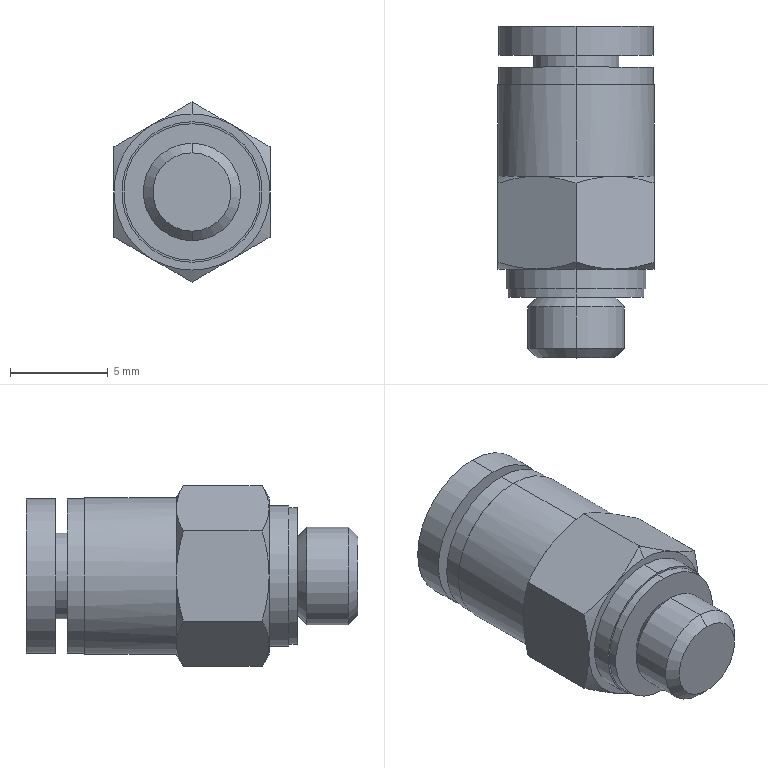Part | SolidWorks | features BaseBody 1 | 1 solid | 49 faces | box 8 x 17 x 9.238 mm | volume 564.577 mm3 | cone 18 | cylinder 16 | plane 15 | commonest cylinder face diameters 7.9 x4 4.2 x2 4.4 x2 5 x2 7 x2 7.2 x2
STEP:
#1=CARTESIAN_POINT('',(0.,1.2,-2.1));
#2=VERTEX_POINT('',#1);
#3=CARTESIAN_POINT('',(0.,1.2,2.1));
#4=VERTEX_POINT('',#3);
#5=CARTESIAN_POINT('',(0.,1.2,0.));
#6=DIRECTION('',(0.,1.,0.));
#7=DIRECTION('',(0.,0.,1.));
#8=AXIS2_PLACEMENT_3D('',#5,#6,#7);
#9=CIRCLE('',#8,2.1);
#10=EDGE_CURVE('',#2,#4,#9,.T.);
#11=ORIENTED_EDGE('',*,*,#10,.F.);
#12=CARTESIAN_POINT('',(0.,13.9,-2.1));
#13=VERTEX_POINT('',#12);
#14=CARTESIAN_POINT('',(0.,7.55,-2.1));
#15=DIRECTION('',(0.,1.,0.));
#16=VECTOR('',#15,1000.);
#17=LINE('',#14,#16);
#18=EDGE_CURVE('',#2,#13,#17,.T.);
#19=ORIENTED_EDGE('',*,*,#18,.T.);
#20=CARTESIAN_POINT('',(0.,13.9,2.1));
#21=VERTEX_POINT('',#20);
#22=CARTESIAN_POINT('',(0.,13.9,0.));
#23=DIRECTION('',(0.,-1.,0.));
#24=DIRECTION('',(0.,0.,1.));
#25=AXIS2_PLACEMENT_3D('',#22,#23,#24);
#26=CIRCLE('',#25,2.1);
#27=EDGE_CURVE('',#21,#13,#26,.T.);
#28=ORIENTED_EDGE('',*,*,#27,.F.);
#29=CARTESIAN_POINT('',(0.,7.55,2.1));
#30=DIRECTION('',(0.,1.,0.));
#31=VECTOR('',#30,1000.);
#32=LINE('',#29,#31);
#33=EDGE_CURVE('',#4,#21,#32,.T.);
#34=ORIENTED_EDGE('',*,*,#33,.F.);
#35=EDGE_LOOP('',(#11,#19,#28,#34));
#36=FACE_OUTER_BOUND('',#35,.T.);
#37=CARTESIAN_POINT('',(0.,7.55,0.));
#38=DIRECTION('',(0.,1.,0.));
#39=DIRECTION('',(0.,0.,1.));
#40=AXIS2_PLACEMENT_3D('',#37,#38,#39);
#41=CYLINDRICAL_SURFACE('',#40,2.1);
#42=ADVANCED_FACE('',(#36),#41,.F.);
#43=CARTESIAN_POINT('',(0.,12.4,3.95));
#44=VERTEX_POINT('',#43);
#45=CARTESIAN_POINT('',(0.,12.4,-3.95));
#46=VERTEX_POINT('',#45);
#47=CARTESIAN_POINT('',(0.,12.4,0.));
#48=DIRECTION('',(0.,1.,0.));
#49=DIRECTION('',(0.,0.,1.));
#50=AXIS2_PLACEMENT_3D('',#47,#48,#49);
#51=CIRCLE('',#50,3.95);
#52=EDGE_CURVE('',#44,#46,#51,.T.);
#53=ORIENTED_EDGE('',*,*,#52,.T.);
#54=CARTESIAN_POINT('',(0.,13.9,-3.95));
#55=VERTEX_POINT('',#54);
#56=CARTESIAN_POINT('',(0.,13.15,-3.95));
#57=DIRECTION('',(0.,1.,0.));
#58=VECTOR('',#57,1000.);
#59=LINE('',#56,#58);
#60=EDGE_CURVE('',#46,#55,#59,.T.);
#61=ORIENTED_EDGE('',*,*,#60,.T.);
#62=CARTESIAN_POINT('',(0.,13.9,3.95));
#63=VERTEX_POINT('',#62);
#64=CARTESIAN_POINT('',(0.,13.9,0.));
#65=DIRECTION('',(0.,1.,0.));
#66=DIRECTION('',(0.,0.,1.));
#67=AXIS2_PLACEMENT_3D('',#64,#65,#66);
#68=CIRCLE('',#67,3.95);
#69=EDGE_CURVE('',#63,#55,#68,.T.);
#70=ORIENTED_EDGE('',*,*,#69,.F.);
#71=CARTESIAN_POINT('',(0.,13.15,3.95));
#72=DIRECTION('',(0.,1.,0.));
#73=VECTOR('',#72,1000.);
#74=LINE('',#71,#73);
#75=EDGE_CURVE('',#44,#63,#74,.T.);
#76=ORIENTED_EDGE('',*,*,#75,.F.);
#77=EDGE_LOOP('',(#53,#61,#70,#76));
#78=FACE_OUTER_BOUND('',#77,.T.);
#79=CARTESIAN_POINT('',(0.,13.15,0.));
#80=DIRECTION('',(0.,1.,0.));
#81=DIRECTION('',(0.,0.,1.));
#82=AXIS2_PLACEMENT_3D('',#79,#80,#81);
#83=CYLINDRICAL_SURFACE('',#82,3.95);
#84=ADVANCED_FACE('',(#78),#83,.T.);
#85=CARTESIAN_POINT('',(0.,11.8,2.2));
#86=VERTEX_POINT('',#85);
#87=CARTESIAN_POINT('',(0.,11.8,-2.2));
#88=VERTEX_POINT('',#87);
#89=CARTESIAN_POINT('',(0.,11.8,0.));
#90=DIRECTION('',(0.,1.,0.));
#91=DIRECTION('',(0.,0.,1.));
#92=AXIS2_PLACEMENT_3D('',#89,#90,#91);
#93=CIRCLE('',#92,2.2);
#94=EDGE_CURVE('',#86,#88,#93,.T.);
#95=ORIENTED_EDGE('',*,*,#94,.T.);
#96=CARTESIAN_POINT('',(0.,12.4,-2.2));
#97=VERTEX_POINT('',#96);
#98=CARTESIAN_POINT('',(0.,12.1,-2.2));
#99=DIRECTION('',(0.,1.,0.));
#100=VECTOR('',#99,1000.);
#101=LINE('',#98,#100);
#102=EDGE_CURVE('',#88,#97,#101,.T.);
#103=ORIENTED_EDGE('',*,*,#102,.T.);
#104=CARTESIAN_POINT('',(0.,12.4,2.2));
#105=VERTEX_POINT('',#104);
#106=CARTESIAN_POINT('',(0.,12.4,0.));
#107=DIRECTION('',(0.,1.,0.));
#108=DIRECTION('',(0.,0.,1.));
#109=AXIS2_PLACEMENT_3D('',#106,#107,#108);
#110=CIRCLE('',#109,2.2);
#111=EDGE_CURVE('',#105,#97,#110,.T.);
#112=ORIENTED_EDGE('',*,*,#111,.F.);
#113=CARTESIAN_POINT('',(0.,12.1,2.2));
#114=DIRECTION('',(0.,1.,0.));
#115=VECTOR('',#114,1000.);
#116=LINE('',#113,#115);
#117=EDGE_CURVE('',#86,#105,#116,.T.);
#118=ORIENTED_EDGE('',*,*,#117,.F.);
#119=EDGE_LOOP('',(#95,#103,#112,#118));
#120=FACE_OUTER_BOUND('',#119,.T.);
#121=CARTESIAN_POINT('',(0.,12.1,0.));
#122=DIRECTION('',(0.,1.,0.));
#123=DIRECTION('',(0.,0.,1.));
#124=AXIS2_PLACEMENT_3D('',#121,#122,#123);
#125=CYLINDRICAL_SURFACE('',#124,2.2);
#126=ADVANCED_FACE('',(#120),#125,.T.);
#127=CARTESIAN_POINT('',(0.,10.9,3.95));
#128=VERTEX_POINT('',#127);
#129=CARTESIAN_POINT('',(0.,10.9,-3.95));
#130=VERTEX_POINT('',#129);
#131=CARTESIAN_POINT('',(0.,10.9,0.));
#132=DIRECTION('',(0.,1.,0.));
#133=DIRECTION('',(0.,0.,1.));
#134=AXIS2_PLACEMENT_3D('',#131,#132,#133);
#135=CIRCLE('',#134,3.95);
#136=EDGE_CURVE('',#128,#130,#135,.T.);
#137=ORIENTED_EDGE('',*,*,#136,.T.);
#138=CARTESIAN_POINT('',(0.,11.8,-3.95));
#139=VERTEX_POINT('',#138);
#140=CARTESIAN_POINT('',(0.,11.35,-3.95));
#141=DIRECTION('',(0.,1.,0.));
#142=VECTOR('',#141,1000.);
#143=LINE('',#140,#142);
#144=EDGE_CURVE('',#130,#139,#143,.T.);
#145=ORIENTED_EDGE('',*,*,#144,.T.);
#146=CARTESIAN_POINT('',(0.,11.8,3.95));
#147=VERTEX_POINT('',#146);
#148=CARTESIAN_POINT('',(0.,11.8,0.));
#149=DIRECTION('',(0.,1.,0.));
#150=DIRECTION('',(0.,0.,1.));
#151=AXIS2_PLACEMENT_3D('',#148,#149,#150);
#152=CIRCLE('',#151,3.95);
#153=EDGE_CURVE('',#147,#139,#152,.T.);
#154=ORIENTED_EDGE('',*,*,#153,.F.);
#155=CARTESIAN_POINT('',(0.,11.35,3.95));
#156=DIRECTION('',(0.,1.,0.));
#157=VECTOR('',#156,1000.);
#158=LINE('',#155,#157);
#159=EDGE_CURVE('',#128,#147,#158,.T.);
#160=ORIENTED_EDGE('',*,*,#159,.F.);
#161=EDGE_LOOP('',(#137,#145,#154,#160));
#162=FACE_OUTER_BOUND('',#161,.T.);
#163=CARTESIAN_POINT('',(0.,11.35,0.));
#164=DIRECTION('',(0.,1.,0.));
#165=DIRECTION('',(0.,0.,1.));
#166=AXIS2_PLACEMENT_3D('',#163,#164,#165);
#167=CYLINDRICAL_SURFACE('',#166,3.95);
#168=ADVANCED_FACE('',(#162),#167,.T.);
#169=CARTESIAN_POINT('',(2.,6.2,-3.464));
#170=VERTEX_POINT('',#169);
#171=CARTESIAN_POINT('',(0.,6.2,-4.));
#172=VERTEX_POINT('',#171);
#173=CARTESIAN_POINT('',(0.,6.2,0.));
#174=DIRECTION('',(0.,1.,0.));
#175=DIRECTION('',(0.,0.,1.));
#176=AXIS2_PLACEMENT_3D('',#173,#174,#175);
#177=CIRCLE('',#176,4.);
#178=EDGE_CURVE('',#170,#172,#177,.T.);
#179=ORIENTED_EDGE('',*,*,#178,.T.);
#180=CARTESIAN_POINT('',(0.,10.9,-4.));
#181=VERTEX_POINT('',#180);
#182=CARTESIAN_POINT('',(0.,8.55,-4.));
#183=DIRECTION('',(0.,1.,0.));
#184=VECTOR('',#183,1000.);
#185=LINE('',#182,#184);
#186=EDGE_CURVE('',#172,#181,#185,.T.);
#187=ORIENTED_EDGE('',*,*,#186,.T.);
#188=CARTESIAN_POINT('',(0.,10.9,4.));
#189=VERTEX_POINT('',#188);
#190=CARTESIAN_POINT('',(0.,10.9,0.));
#191=DIRECTION('',(0.,1.,0.));
#192=DIRECTION('',(0.,0.,1.));
#193=AXIS2_PLACEMENT_3D('',#190,#191,#192);
#194=CIRCLE('',#193,4.);
#195=EDGE_CURVE('',#189,#181,#194,.T.);
#196=ORIENTED_EDGE('',*,*,#195,.F.);
#197=CARTESIAN_POINT('',(0.,6.2,4.));
#198=VERTEX_POINT('',#197);
#199=CARTESIAN_POINT('',(0.,8.55,4.));
#200=DIRECTION('',(0.,1.,0.));
#201=VECTOR('',#200,1000.);
#202=LINE('',#199,#201);
#203=EDGE_CURVE('',#198,#189,#202,.T.);
#204=ORIENTED_EDGE('',*,*,#203,.F.);
#205=CARTESIAN_POINT('',(2.,6.2,3.464));
#206=VERTEX_POINT('',#205);
#207=CARTESIAN_POINT('',(0.,6.2,0.));
#208=DIRECTION('',(0.,1.,0.));
#209=DIRECTION('',(0.,0.,1.));
#210=AXIS2_PLACEMENT_3D('',#207,#208,#209);
#211=CIRCLE('',#210,4.);
#212=EDGE_CURVE('',#198,#206,#211,.T.);
#213=ORIENTED_EDGE('',*,*,#212,.T.);
#214=CARTESIAN_POINT('',(4.,6.2,0.));
#215=VERTEX_POINT('',#214);
#216=CARTESIAN_POINT('',(0.,6.2,0.));
#217=DIRECTION('',(0.,1.,0.));
#218=DIRECTION('',(0.,0.,1.));
#219=AXIS2_PLACEMENT_3D('',#216,#217,#218);
#220=CIRCLE('',#219,4.);
#221=EDGE_CURVE('',#206,#215,#220,.T.);
#222=ORIENTED_EDGE('',*,*,#221,.T.);
#223=CARTESIAN_POINT('',(0.,6.2,0.));
#224=DIRECTION('',(0.,1.,0.));
#225=DIRECTION('',(0.,0.,1.));
#226=AXIS2_PLACEMENT_3D('',#223,#224,#225);
#227=CIRCLE('',#226,4.);
#228=EDGE_CURVE('',#215,#170,#227,.T.);
#229=ORIENTED_EDGE('',*,*,#228,.T.);
#230=EDGE_LOOP('',(#179,#187,#196,#204,#213,#222,#229));
#231=FACE_OUTER_BOUND('',#230,.T.);
#232=CARTESIAN_POINT('',(0.,8.55,0.));
#233=DIRECTION('',(0.,1.,0.));
#234=DIRECTION('',(0.,0.,1.));
#235=AXIS2_PLACEMENT_3D('',#232,#233,#234);
#236=CYLINDRICAL_SURFACE('',#235,4.);
#237=ADVANCED_FACE('',(#231),#236,.T.);
#238=CARTESIAN_POINT('',(-2.,6.2,-3.464));
#239=VERTEX_POINT('',#238);
#240=CARTESIAN_POINT('',(0.,6.2,0.));
#241=DIRECTION('',(0.,1.,0.));
#242=DIRECTION('',(0.,0.,1.));
#243=AXIS2_PLACEMENT_3D('',#240,#241,#242);
#244=CIRCLE('',#243,4.);
#245=EDGE_CURVE('',#172,#239,#244,.T.);
#246=ORIENTED_EDGE('',*,*,#245,.F.);
#247=CARTESIAN_POINT('',(0.,5.843,-4.619));
#248=VERTEX_POINT('',#247);
#249=CARTESIAN_POINT('',(0.,5.841,-4.623));
#250=DIRECTION('',(0.,-0.5,-0.866));
#251=VECTOR('',#250,1000.);
#252=LINE('',#249,#251);
#253=EDGE_CURVE('',#172,#248,#252,.T.);
#254=ORIENTED_EDGE('',*,*,#253,.T.);
#255=CARTESIAN_POINT('',(0.,5.843,-4.619));
#256=CARTESIAN_POINT('',(-0.6534,6.061,-4.242));
#257=CARTESIAN_POINT('',(-1.317,6.2,-3.858));
#258=CARTESIAN_POINT('',(-2.,6.2,-3.464));
#259=B_SPLINE_CURVE_WITH_KNOTS('',3,(#255,#256,#257,#258),.UNSPECIFIED.,.F.,.F.,(4,4),(0.,0.002337),.UNSPECIFIED.);
#260=EDGE_CURVE('',#248,#239,#259,.T.);
#261=ORIENTED_EDGE('',*,*,#260,.T.);
#262=EDGE_LOOP('',(#246,#254,#261));
#263=FACE_OUTER_BOUND('',#262,.T.);
#264=CARTESIAN_POINT('',(0.,5.841,0.));
#265=DIRECTION('',(0.,-1.,0.));
#266=DIRECTION('',(0.,0.,-1.));
#267=AXIS2_PLACEMENT_3D('',#264,#265,#266);
#268=CONICAL_SURFACE('',#267,4.623,1.047);
#269=ADVANCED_FACE('',(#263),#268,.T.);
#270=CARTESIAN_POINT('',(-2.,1.45,3.464));
#271=VERTEX_POINT('',#270);
#272=CARTESIAN_POINT('',(0.,1.45,4.));
#273=VERTEX_POINT('',#272);
#274=CARTESIAN_POINT('',(0.,1.45,0.));
#275=DIRECTION('',(0.,1.,0.));
#276=DIRECTION('',(0.,0.,1.));
#277=AXIS2_PLACEMENT_3D('',#274,#275,#276);
#278=CIRCLE('',#277,4.);
#279=EDGE_CURVE('',#271,#273,#278,.T.);
#280=ORIENTED_EDGE('',*,*,#279,.T.);
#281=CARTESIAN_POINT('',(0.,1.807,4.619));
#282=VERTEX_POINT('',#281);
#283=CARTESIAN_POINT('',(0.,1.809,4.623));
#284=DIRECTION('',(0.,0.5,0.866));
#285=VECTOR('',#284,1000.);
#286=LINE('',#283,#285);
#287=EDGE_CURVE('',#273,#282,#286,.T.);
#288=ORIENTED_EDGE('',*,*,#287,.T.);
#289=CARTESIAN_POINT('',(0.,1.807,4.619));
#290=CARTESIAN_POINT('',(-0.6534,1.589,4.242));
#291=CARTESIAN_POINT('',(-1.317,1.45,3.858));
#292=CARTESIAN_POINT('',(-2.,1.45,3.464));
#293=B_SPLINE_CURVE_WITH_KNOTS('',3,(#289,#290,#291,#292),.UNSPECIFIED.,.F.,.F.,(4,4),(0.,0.002337),.UNSPECIFIED.);
#294=EDGE_CURVE('',#282,#271,#293,.T.);
#295=ORIENTED_EDGE('',*,*,#294,.T.);
#296=EDGE_LOOP('',(#280,#288,#295));
#297=FACE_OUTER_BOUND('',#296,.T.);
#298=CARTESIAN_POINT('',(0.,1.809,0.));
#299=DIRECTION('',(0.,1.,0.));
#300=DIRECTION('',(0.,0.,1.));
#301=AXIS2_PLACEMENT_3D('',#298,#299,#300);
#302=CONICAL_SURFACE('',#301,4.623,1.047);
#303=ADVANCED_FACE('',(#297),#302,.T.);
#304=CARTESIAN_POINT('',(0.,0.45,3.6));
#305=VERTEX_POINT('',#304);
#306=CARTESIAN_POINT('',(0.,0.45,-3.6));
#307=VERTEX_POINT('',#306);
#308=CARTESIAN_POINT('',(0.,0.45,0.));
#309=DIRECTION('',(0.,1.,0.));
#310=DIRECTION('',(0.,0.,1.));
#311=AXIS2_PLACEMENT_3D('',#308,#309,#310);
#312=CIRCLE('',#311,3.6);
#313=EDGE_CURVE('',#305,#307,#312,.T.);
#314=ORIENTED_EDGE('',*,*,#313,.T.);
#315=CARTESIAN_POINT('',(0.,1.45,-3.6));
#316=VERTEX_POINT('',#315);
#317=CARTESIAN_POINT('',(0.,0.95,-3.6));
#318=DIRECTION('',(0.,1.,0.));
#319=VECTOR('',#318,1000.);
#320=LINE('',#317,#319);
#321=EDGE_CURVE('',#307,#316,#320,.T.);
#322=ORIENTED_EDGE('',*,*,#321,.T.);
#323=CARTESIAN_POINT('',(0.,1.45,3.6));
#324=VERTEX_POINT('',#323);
#325=CARTESIAN_POINT('',(0.,1.45,0.));
#326=DIRECTION('',(0.,1.,0.));
#327=DIRECTION('',(0.,0.,1.));
#328=AXIS2_PLACEMENT_3D('',#325,#326,#327);
#329=CIRCLE('',#328,3.6);
#330=EDGE_CURVE('',#324,#316,#329,.T.);
#331=ORIENTED_EDGE('',*,*,#330,.F.);
#332=CARTESIAN_POINT('',(0.,0.95,3.6));
#333=DIRECTION('',(0.,1.,0.));
#334=VECTOR('',#333,1000.);
#335=LINE('',#332,#334);
#336=EDGE_CURVE('',#305,#324,#335,.T.);
#337=ORIENTED_EDGE('',*,*,#336,.F.);
#338=EDGE_LOOP('',(#314,#322,#331,#337));
#339=FACE_OUTER_BOUND('',#338,.T.);
#340=CARTESIAN_POINT('',(0.,0.95,0.));
#341=DIRECTION('',(0.,1.,0.));
#342=DIRECTION('',(0.,0.,1.));
#343=AXIS2_PLACEMENT_3D('',#340,#341,#342);
#344=CYLINDRICAL_SURFACE('',#343,3.6);
#345=ADVANCED_FACE('',(#339),#344,.T.);
#346=CARTESIAN_POINT('',(0.,0.,3.5));
#347=VERTEX_POINT('',#346);
#348=CARTESIAN_POINT('',(0.,0.,-3.5));
#349=VERTEX_POINT('',#348);
#350=CARTESIAN_POINT('',(0.,0.,0.));
#351=DIRECTION('',(0.,1.,0.));
#352=DIRECTION('',(0.,0.,1.));
#353=AXIS2_PLACEMENT_3D('',#350,#351,#352);
#354=CIRCLE('',#353,3.5);
#355=EDGE_CURVE('',#347,#349,#354,.T.);
#356=ORIENTED_EDGE('',*,*,#355,.T.);
#357=CARTESIAN_POINT('',(0.,0.45,-3.5));
#358=VERTEX_POINT('',#357);
#359=CARTESIAN_POINT('',(0.,0.225,-3.5));
#360=DIRECTION('',(0.,1.,0.));
#361=VECTOR('',#360,1000.);
#362=LINE('',#359,#361);
#363=EDGE_CURVE('',#349,#358,#362,.T.);
#364=ORIENTED_EDGE('',*,*,#363,.T.);
#365=CARTESIAN_POINT('',(0.,0.45,3.5));
#366=VERTEX_POINT('',#365);
#367=CARTESIAN_POINT('',(0.,0.45,0.));
#368=DIRECTION('',(0.,1.,0.));
#369=DIRECTION('',(0.,0.,1.));
#370=AXIS2_PLACEMENT_3D('',#367,#368,#369);
#371=CIRCLE('',#370,3.5);
#372=EDGE_CURVE('',#366,#358,#371,.T.);
#373=ORIENTED_EDGE('',*,*,#372,.F.);
#374=CARTESIAN_POINT('',(0.,0.225,3.5));
#375=DIRECTION('',(0.,1.,0.));
#376=VECTOR('',#375,1000.);
#377=LINE('',#374,#376);
#378=EDGE_CURVE('',#347,#366,#377,.T.);
#379=ORIENTED_EDGE('',*,*,#378,.F.);
#380=EDGE_LOOP('',(#356,#364,#373,#379));
#381=FACE_OUTER_BOUND('',#380,.T.);
#382=CARTESIAN_POINT('',(0.,0.225,0.));
#383=DIRECTION('',(0.,1.,0.));
#384=DIRECTION('',(0.,0.,1.));
#385=AXIS2_PLACEMENT_3D('',#382,#383,#384);
#386=CYLINDRICAL_SURFACE('',#385,3.5);
#387=ADVANCED_FACE('',(#381),#386,.T.);
#388=CARTESIAN_POINT('',(0.,0.,2.01));
#389=VERTEX_POINT('',#388);
#390=CARTESIAN_POINT('',(0.,0.,-2.01));
#391=VERTEX_POINT('',#390);
#392=CARTESIAN_POINT('',(0.,0.,0.));
#393=DIRECTION('',(0.,1.,0.));
#394=DIRECTION('',(0.,0.,-1.));
#395=AXIS2_PLACEMENT_3D('',#392,#393,#394);
#396=CIRCLE('',#395,2.01);
#397=EDGE_CURVE('',#389,#391,#396,.T.);
#398=ORIENTED_EDGE('',*,*,#397,.F.);
#399=CARTESIAN_POINT('',(0.,-0.4905,2.5));
#400=VERTEX_POINT('',#399);
#401=CARTESIAN_POINT('',(0.,-0.4905,2.5));
#402=DIRECTION('',(0.,-0.7071,0.7071));
#403=VECTOR('',#402,1000.);
#404=LINE('',#401,#403);
#405=EDGE_CURVE('',#389,#400,#404,.T.);
#406=ORIENTED_EDGE('',*,*,#405,.T.);
#407=CARTESIAN_POINT('',(0.,-0.4905,-2.5));
#408=VERTEX_POINT('',#407);
#409=CARTESIAN_POINT('',(0.,-0.4905,0.));
#410=DIRECTION('',(0.,1.,0.));
#411=DIRECTION('',(0.,0.,1.));
#412=AXIS2_PLACEMENT_3D('',#409,#410,#411);
#413=CIRCLE('',#412,2.5);
#414=EDGE_CURVE('',#400,#408,#413,.T.);
#415=ORIENTED_EDGE('',*,*,#414,.T.);
#416=CARTESIAN_POINT('',(0.,-0.4905,-2.5));
#417=DIRECTION('',(0.,-0.7071,-0.7071));
#418=VECTOR('',#417,1000.);
#419=LINE('',#416,#418);
#420=EDGE_CURVE('',#391,#408,#419,.T.);
#421=ORIENTED_EDGE('',*,*,#420,.F.);
#422=EDGE_LOOP('',(#398,#406,#415,#421));
#423=FACE_OUTER_BOUND('',#422,.T.);
#424=CARTESIAN_POINT('',(0.,-0.4905,0.));
#425=DIRECTION('',(0.,-1.,0.));
#426=DIRECTION('',(0.,0.,-1.));
#427=AXIS2_PLACEMENT_3D('',#424,#425,#426);
#428=CONICAL_SURFACE('',#427,2.5,0.7854);
#429=ADVANCED_FACE('',(#423),#428,.T.);
#430=CARTESIAN_POINT('',(0.,-2.61,2.5));
#431=VERTEX_POINT('',#430);
#432=CARTESIAN_POINT('',(0.,-2.609,-2.5));
#433=VERTEX_POINT('',#432);
#434=CARTESIAN_POINT('',(0.,-2.609,0.));
#435=DIRECTION('',(0.,1.,0.));
#436=DIRECTION('',(0.,0.,1.));
#437=AXIS2_PLACEMENT_3D('',#434,#435,#436);
#438=CIRCLE('',#437,2.5);
#439=EDGE_CURVE('',#431,#433,#438,.T.);
#440=ORIENTED_EDGE('',*,*,#439,.T.);
#441=CARTESIAN_POINT('',(0.,-1.55,-2.5));
#442=DIRECTION('',(0.,1.,0.));
#443=VECTOR('',#442,1000.);
#444=LINE('',#441,#443);
#445=EDGE_CURVE('',#433,#408,#444,.T.);
#446=ORIENTED_EDGE('',*,*,#445,.T.);
#447=ORIENTED_EDGE('',*,*,#414,.F.);
#448=CARTESIAN_POINT('',(0.,-1.55,2.5));
#449=DIRECTION('',(0.,1.,0.));
#450=VECTOR('',#449,1000.);
#451=LINE('',#448,#450);
#452=EDGE_CURVE('',#431,#400,#451,.T.);
#453=ORIENTED_EDGE('',*,*,#452,.F.);
#454=EDGE_LOOP('',(#440,#446,#447,#453));
#455=FACE_OUTER_BOUND('',#454,.T.);
#456=CARTESIAN_POINT('',(0.,-1.55,0.));
#457=DIRECTION('',(0.,1.,0.));
#458=DIRECTION('',(0.,0.,1.));
#459=AXIS2_PLACEMENT_3D('',#456,#457,#458);
#460=CYLINDRICAL_SURFACE('',#459,2.5);
#461=ADVANCED_FACE('',(#455),#460,.T.);
#462=CARTESIAN_POINT('',(0.,-3.1,2.009));
#463=VERTEX_POINT('',#462);
#464=CARTESIAN_POINT('',(0.,-3.1,-2.009));
#465=VERTEX_POINT('',#464);
#466=CARTESIAN_POINT('',(0.,-3.1,0.));
#467=DIRECTION('',(0.,1.,0.));
#468=DIRECTION('',(0.,0.,1.));
#469=AXIS2_PLACEMENT_3D('',#466,#467,#468);
#470=CIRCLE('',#469,2.009);
#471=EDGE_CURVE('',#463,#465,#470,.T.);
#472=ORIENTED_EDGE('',*,*,#471,.T.);
#473=CARTESIAN_POINT('',(0.,-2.61,-2.5));
#474=DIRECTION('',(0.,0.7071,-0.7071));
#475=VECTOR('',#474,1000.);
#476=LINE('',#473,#475);
#477=EDGE_CURVE('',#465,#433,#476,.T.);
#478=ORIENTED_EDGE('',*,*,#477,.T.);
#479=ORIENTED_EDGE('',*,*,#439,.F.);
#480=CARTESIAN_POINT('',(0.,-2.61,2.5));
#481=DIRECTION('',(0.,0.7071,0.7071));
#482=VECTOR('',#481,1000.);
#483=LINE('',#480,#482);
#484=EDGE_CURVE('',#463,#431,#483,.T.);
#485=ORIENTED_EDGE('',*,*,#484,.F.);
#486=EDGE_LOOP('',(#472,#478,#479,#485));
#487=FACE_OUTER_BOUND('',#486,.T.);
#488=CARTESIAN_POINT('',(0.,-2.61,0.));
#489=DIRECTION('',(0.,1.,0.));
#490=DIRECTION('',(0.,0.,1.));
#491=AXIS2_PLACEMENT_3D('',#488,#489,#490);
#492=CONICAL_SURFACE('',#491,2.5,0.7854);
#493=ADVANCED_FACE('',(#487),#492,.T.);
#494=ORIENTED_EDGE('',*,*,#18,.F.);
#495=CARTESIAN_POINT('',(0.,1.2,0.));
#496=DIRECTION('',(0.,1.,0.));
#497=DIRECTION('',(0.,0.,1.));
#498=AXIS2_PLACEMENT_3D('',#495,#496,#497);
#499=CIRCLE('',#498,2.1);
#500=EDGE_CURVE('',#4,#2,#499,.T.);
#501=ORIENTED_EDGE('',*,*,#500,.F.);
#502=ORIENTED_EDGE('',*,*,#33,.T.);
#503=CARTESIAN_POINT('',(0.,13.9,0.));
#504=DIRECTION('',(0.,-1.,0.));
#505=DIRECTION('',(0.,0.,1.));
#506=AXIS2_PLACEMENT_3D('',#503,#504,#505);
#507=CIRCLE('',#506,2.1);
#508=EDGE_CURVE('',#13,#21,#507,.T.);
#509=ORIENTED_EDGE('',*,*,#508,.F.);
#510=EDGE_LOOP('',(#494,#501,#502,#509));
#511=FACE_OUTER_BOUND('',#510,.T.);
#512=CARTESIAN_POINT('',(0.,7.55,0.));
#513=DIRECTION('',(0.,1.,0.));
#514=DIRECTION('',(0.,0.,1.));
#515=AXIS2_PLACEMENT_3D('',#512,#513,#514);
#516=CYLINDRICAL_SURFACE('',#515,2.1);
#517=ADVANCED_FACE('',(#511),#516,.F.);
#518=ORIENTED_EDGE('',*,*,#27,.T.);
#519=ORIENTED_EDGE('',*,*,#508,.T.);
#520=EDGE_LOOP('',(#518,#519));
#521=FACE_BOUND('',#520,.T.);
#522=ORIENTED_EDGE('',*,*,#69,.T.);
#523=CARTESIAN_POINT('',(0.,13.9,0.));
#524=DIRECTION('',(0.,1.,0.));
#525=DIRECTION('',(0.,0.,1.));
#526=AXIS2_PLACEMENT_3D('',#523,#524,#525);
#527=CIRCLE('',#526,3.95);
#528=EDGE_CURVE('',#55,#63,#527,.T.);
#529=ORIENTED_EDGE('',*,*,#528,.T.);
#530=EDGE_LOOP('',(#522,#529));
#531=FACE_OUTER_BOUND('',#530,.T.);
#532=CARTESIAN_POINT('',(0.,13.9,3.025));
#533=DIRECTION('',(0.,1.,0.));
#534=DIRECTION('',(-1.,0.,0.));
#535=AXIS2_PLACEMENT_3D('',#532,#533,#534);
#536=PLANE('',#535);
#537=ADVANCED_FACE('',(#521,#531),#536,.T.);
#538=ORIENTED_EDGE('',*,*,#500,.T.);
#539=ORIENTED_EDGE('',*,*,#10,.T.);
#540=EDGE_LOOP('',(#538,#539));
#541=FACE_OUTER_BOUND('',#540,.T.);
#542=CARTESIAN_POINT('',(0.,1.2,1.05));
#543=DIRECTION('',(0.,1.,0.));
#544=DIRECTION('',(0.,0.,1.));
#545=AXIS2_PLACEMENT_3D('',#542,#543,#544);
#546=PLANE('',#545);
#547=ADVANCED_FACE('',(#541),#546,.T.);
#548=ORIENTED_EDGE('',*,*,#60,.F.);
#549=CARTESIAN_POINT('',(0.,12.4,0.));
#550=DIRECTION('',(0.,1.,0.));
#551=DIRECTION('',(0.,0.,1.));
#552=AXIS2_PLACEMENT_3D('',#549,#550,#551);
#553=CIRCLE('',#552,3.95);
#554=EDGE_CURVE('',#46,#44,#553,.T.);
#555=ORIENTED_EDGE('',*,*,#554,.T.);
#556=ORIENTED_EDGE('',*,*,#75,.T.);
#557=ORIENTED_EDGE('',*,*,#528,.F.);
#558=EDGE_LOOP('',(#548,#555,#556,#557));
#559=FACE_OUTER_BOUND('',#558,.T.);
#560=CARTESIAN_POINT('',(0.,13.15,0.));
#561=DIRECTION('',(0.,1.,0.));
#562=DIRECTION('',(0.,0.,1.));
#563=AXIS2_PLACEMENT_3D('',#560,#561,#562);
#564=CYLINDRICAL_SURFACE('',#563,3.95);
#565=ADVANCED_FACE('',(#559),#564,.T.);
#566=ORIENTED_EDGE('',*,*,#52,.F.);
#567=ORIENTED_EDGE('',*,*,#554,.F.);
#568=EDGE_LOOP('',(#566,#567));
#569=FACE_OUTER_BOUND('',#568,.T.);
#570=ORIENTED_EDGE('',*,*,#111,.T.);
#571=CARTESIAN_POINT('',(0.,12.4,0.));
#572=DIRECTION('',(0.,1.,0.));
#573=DIRECTION('',(0.,0.,1.));
#574=AXIS2_PLACEMENT_3D('',#571,#572,#573);
#575=CIRCLE('',#574,2.2);
#576=EDGE_CURVE('',#97,#105,#575,.T.);
#577=ORIENTED_EDGE('',*,*,#576,.T.);
#578=EDGE_LOOP('',(#570,#577));
#579=FACE_BOUND('',#578,.T.);
#580=CARTESIAN_POINT('',(0.,12.4,3.075));
#581=DIRECTION('',(0.,-1.,0.));
#582=DIRECTION('',(1.,0.,0.));
#583=AXIS2_PLACEMENT_3D('',#580,#581,#582);
#584=PLANE('',#583);
#585=ADVANCED_FACE('',(#569,#579),#584,.T.);
#586=ORIENTED_EDGE('',*,*,#102,.F.);
#587=CARTESIAN_POINT('',(0.,11.8,0.));
#588=DIRECTION('',(0.,1.,0.));
#589=DIRECTION('',(0.,0.,1.));
#590=AXIS2_PLACEMENT_3D('',#587,#588,#589);
#591=CIRCLE('',#590,2.2);
#592=EDGE_CURVE('',#88,#86,#591,.T.);
#593=ORIENTED_EDGE('',*,*,#592,.T.);
#594=ORIENTED_EDGE('',*,*,#117,.T.);
#595=ORIENTED_EDGE('',*,*,#576,.F.);
#596=EDGE_LOOP('',(#586,#593,#594,#595));
#597=FACE_OUTER_BOUND('',#596,.T.);
#598=CARTESIAN_POINT('',(0.,12.1,0.));
#599=DIRECTION('',(0.,1.,0.));
#600=DIRECTION('',(0.,0.,1.));
#601=AXIS2_PLACEMENT_3D('',#598,#599,#600);
#602=CYLINDRICAL_SURFACE('',#601,2.2);
#603=ADVANCED_FACE('',(#597),#602,.T.);
#604=ORIENTED_EDGE('',*,*,#94,.F.);
#605=ORIENTED_EDGE('',*,*,#592,.F.);
#606=EDGE_LOOP('',(#604,#605));
#607=FACE_BOUND('',#606,.T.);
#608=ORIENTED_EDGE('',*,*,#153,.T.);
#609=CARTESIAN_POINT('',(0.,11.8,0.));
#610=DIRECTION('',(0.,1.,0.));
#611=DIRECTION('',(0.,0.,1.));
#612=AXIS2_PLACEMENT_3D('',#609,#610,#611);
#613=CIRCLE('',#612,3.95);
#614=EDGE_CURVE('',#139,#147,#613,.T.);
#615=ORIENTED_EDGE('',*,*,#614,.T.);
#616=EDGE_LOOP('',(#608,#615));
#617=FACE_OUTER_BOUND('',#616,.T.);
#618=CARTESIAN_POINT('',(0.,11.8,3.075));
#619=DIRECTION('',(0.,1.,0.));
#620=DIRECTION('',(-1.,0.,0.));
#621=AXIS2_PLACEMENT_3D('',#618,#619,#620);
#622=PLANE('',#621);
#623=ADVANCED_FACE('',(#607,#617),#622,.T.);
#624=ORIENTED_EDGE('',*,*,#144,.F.);
#625=CARTESIAN_POINT('',(0.,10.9,0.));
#626=DIRECTION('',(0.,1.,0.));
#627=DIRECTION('',(0.,0.,1.));
#628=AXIS2_PLACEMENT_3D('',#625,#626,#627);
#629=CIRCLE('',#628,3.95);
#630=EDGE_CURVE('',#130,#128,#629,.T.);
#631=ORIENTED_EDGE('',*,*,#630,.T.);
#632=ORIENTED_EDGE('',*,*,#159,.T.);
#633=ORIENTED_EDGE('',*,*,#614,.F.);
#634=EDGE_LOOP('',(#624,#631,#632,#633));
#635=FACE_OUTER_BOUND('',#634,.T.);
#636=CARTESIAN_POINT('',(0.,11.35,0.));
#637=DIRECTION('',(0.,1.,0.));
#638=DIRECTION('',(0.,0.,1.));
#639=AXIS2_PLACEMENT_3D('',#636,#637,#638);
#640=CYLINDRICAL_SURFACE('',#639,3.95);
#641=ADVANCED_FACE('',(#635),#640,.T.);
#642=ORIENTED_EDGE('',*,*,#136,.F.);
#643=ORIENTED_EDGE('',*,*,#630,.F.);
#644=EDGE_LOOP('',(#642,#643));
#645=FACE_BOUND('',#644,.T.);
#646=ORIENTED_EDGE('',*,*,#195,.T.);
#647=CARTESIAN_POINT('',(0.,10.9,0.));
#648=DIRECTION('',(0.,1.,0.));
#649=DIRECTION('',(0.,0.,1.));
#650=AXIS2_PLACEMENT_3D('',#647,#648,#649);
#651=CIRCLE('',#650,4.);
#652=EDGE_CURVE('',#181,#189,#651,.T.);
#653=ORIENTED_EDGE('',*,*,#652,.T.);
#654=EDGE_LOOP('',(#646,#653));
#655=FACE_OUTER_BOUND('',#654,.T.);
#656=CARTESIAN_POINT('',(0.,10.9,3.975));
#657=DIRECTION('',(0.,1.,0.));
#658=DIRECTION('',(0.,0.,1.));
#659=AXIS2_PLACEMENT_3D('',#656,#657,#658);
#660=PLANE('',#659);
#661=ADVANCED_FACE('',(#645,#655),#660,.T.);
#662=ORIENTED_EDGE('',*,*,#186,.F.);
#663=ORIENTED_EDGE('',*,*,#245,.T.);
#664=CARTESIAN_POINT('',(-4.,6.2,0.));
#665=VERTEX_POINT('',#664);
#666=CARTESIAN_POINT('',(0.,6.2,0.));
#667=DIRECTION('',(0.,1.,0.));
#668=DIRECTION('',(0.,0.,1.));
#669=AXIS2_PLACEMENT_3D('',#666,#667,#668);
#670=CIRCLE('',#669,4.);
#671=EDGE_CURVE('',#239,#665,#670,.T.);
#672=ORIENTED_EDGE('',*,*,#671,.T.);
#673=CARTESIAN_POINT('',(-2.,6.2,3.464));
#674=VERTEX_POINT('',#673);
#675=CARTESIAN_POINT('',(0.,6.2,0.));
#676=DIRECTION('',(0.,1.,0.));
#677=DIRECTION('',(0.,0.,1.));
#678=AXIS2_PLACEMENT_3D('',#675,#676,#677);
#679=CIRCLE('',#678,4.);
#680=EDGE_CURVE('',#665,#674,#679,.T.);
#681=ORIENTED_EDGE('',*,*,#680,.T.);
#682=CARTESIAN_POINT('',(0.,6.2,0.));
#683=DIRECTION('',(0.,1.,0.));
#684=DIRECTION('',(0.,0.,1.));
#685=AXIS2_PLACEMENT_3D('',#682,#683,#684);
#686=CIRCLE('',#685,4.);
#687=EDGE_CURVE('',#674,#198,#686,.T.);
#688=ORIENTED_EDGE('',*,*,#687,.T.);
#689=ORIENTED_EDGE('',*,*,#203,.T.);
#690=ORIENTED_EDGE('',*,*,#652,.F.);
#691=EDGE_LOOP('',(#662,#663,#672,#681,#688,#689,#690));
#692=FACE_OUTER_BOUND('',#691,.T.);
#693=CARTESIAN_POINT('',(0.,8.55,0.));
#694=DIRECTION('',(0.,1.,0.));
#695=DIRECTION('',(0.,0.,1.));
#696=AXIS2_PLACEMENT_3D('',#693,#694,#695);
#697=CYLINDRICAL_SURFACE('',#696,4.);
#698=ADVANCED_FACE('',(#692),#697,.T.);
#699=ORIENTED_EDGE('',*,*,#253,.F.);
#700=ORIENTED_EDGE('',*,*,#178,.F.);
#701=CARTESIAN_POINT('',(2.,6.2,-3.464));
#702=CARTESIAN_POINT('',(1.317,6.2,-3.858));
#703=CARTESIAN_POINT('',(0.6534,6.061,-4.242));
#704=CARTESIAN_POINT('',(0.,5.843,-4.619));
#705=B_SPLINE_CURVE_WITH_KNOTS('',3,(#701,#702,#703,#704),.UNSPECIFIED.,.F.,.F.,(4,4),(0.,0.002337),.UNSPECIFIED.);
#706=EDGE_CURVE('',#170,#248,#705,.T.);
#707=ORIENTED_EDGE('',*,*,#706,.T.);
#708=EDGE_LOOP('',(#699,#700,#707));
#709=FACE_OUTER_BOUND('',#708,.T.);
#710=CARTESIAN_POINT('',(0.,5.841,0.));
#711=DIRECTION('',(0.,-1.,0.));
#712=DIRECTION('',(0.,0.,-1.));
#713=AXIS2_PLACEMENT_3D('',#710,#711,#712);
#714=CONICAL_SURFACE('',#713,4.623,1.047);
#715=ADVANCED_FACE('',(#709),#714,.T.);
#716=CARTESIAN_POINT('',(4.,5.843,-2.309));
#717=VERTEX_POINT('',#716);
#718=CARTESIAN_POINT('',(4.,5.843,-2.309));
#719=CARTESIAN_POINT('',(3.347,6.061,-2.687));
#720=CARTESIAN_POINT('',(2.683,6.2,-3.07));
#721=CARTESIAN_POINT('',(2.,6.2,-3.464));
#722=B_SPLINE_CURVE_WITH_KNOTS('',3,(#718,#719,#720,#721),.UNSPECIFIED.,.F.,.F.,(4,4),(0.,0.002337),.UNSPECIFIED.);
#723=EDGE_CURVE('',#717,#170,#722,.T.);
#724=ORIENTED_EDGE('',*,*,#723,.T.);
#725=ORIENTED_EDGE('',*,*,#228,.F.);
#726=CARTESIAN_POINT('',(4.,6.2,0.));
#727=CARTESIAN_POINT('',(4.,6.2,-0.7882));
#728=CARTESIAN_POINT('',(4.,6.061,-1.555));
#729=CARTESIAN_POINT('',(4.,5.843,-2.309));
#730=B_SPLINE_CURVE_WITH_KNOTS('',3,(#726,#727,#728,#729),.UNSPECIFIED.,.F.,.F.,(4,4),(0.,0.002337),.UNSPECIFIED.);
#731=EDGE_CURVE('',#215,#717,#730,.T.);
#732=ORIENTED_EDGE('',*,*,#731,.T.);
#733=EDGE_LOOP('',(#724,#725,#732));
#734=FACE_OUTER_BOUND('',#733,.T.);
#735=CARTESIAN_POINT('',(0.,5.841,0.));
#736=DIRECTION('',(0.,-1.,0.));
#737=DIRECTION('',(0.,0.,-1.));
#738=AXIS2_PLACEMENT_3D('',#735,#736,#737);
#739=CONICAL_SURFACE('',#738,4.623,1.047);
#740=ADVANCED_FACE('',(#734),#739,.T.);
#741=CARTESIAN_POINT('',(4.,5.843,2.309));
#742=VERTEX_POINT('',#741);
#743=CARTESIAN_POINT('',(4.,5.843,2.309));
#744=CARTESIAN_POINT('',(4.,6.061,1.555));
#745=CARTESIAN_POINT('',(4.,6.2,0.7882));
#746=CARTESIAN_POINT('',(4.,6.2,0.));
#747=B_SPLINE_CURVE_WITH_KNOTS('',3,(#743,#744,#745,#746),.UNSPECIFIED.,.F.,.F.,(4,4),(0.,0.002337),.UNSPECIFIED.);
#748=EDGE_CURVE('',#742,#215,#747,.T.);
#749=ORIENTED_EDGE('',*,*,#748,.T.);
#750=ORIENTED_EDGE('',*,*,#221,.F.);
#751=CARTESIAN_POINT('',(2.,6.2,3.464));
#752=CARTESIAN_POINT('',(2.683,6.2,3.07));
#753=CARTESIAN_POINT('',(3.347,6.061,2.687));
#754=CARTESIAN_POINT('',(4.,5.843,2.309));
#755=B_SPLINE_CURVE_WITH_KNOTS('',3,(#751,#752,#753,#754),.UNSPECIFIED.,.F.,.F.,(4,4),(0.,0.002337),.UNSPECIFIED.);
#756=EDGE_CURVE('',#206,#742,#755,.T.);
#757=ORIENTED_EDGE('',*,*,#756,.T.);
#758=EDGE_LOOP('',(#749,#750,#757));
#759=FACE_OUTER_BOUND('',#758,.T.);
#760=CARTESIAN_POINT('',(0.,5.841,0.));
#761=DIRECTION('',(0.,-1.,0.));
#762=DIRECTION('',(0.,0.,-1.));
#763=AXIS2_PLACEMENT_3D('',#760,#761,#762);
#764=CONICAL_SURFACE('',#763,4.623,1.047);
#765=ADVANCED_FACE('',(#759),#764,.T.);
#766=CARTESIAN_POINT('',(0.,5.843,4.619));
#767=VERTEX_POINT('',#766);
#768=CARTESIAN_POINT('',(0.,5.843,4.619));
#769=CARTESIAN_POINT('',(0.6534,6.061,4.242));
#770=CARTESIAN_POINT('',(1.317,6.2,3.858));
#771=CARTESIAN_POINT('',(2.,6.2,3.464));
#772=B_SPLINE_CURVE_WITH_KNOTS('',3,(#768,#769,#770,#771),.UNSPECIFIED.,.F.,.F.,(4,4),(0.,0.002337),.UNSPECIFIED.);
#773=EDGE_CURVE('',#767,#206,#772,.T.);
#774=ORIENTED_EDGE('',*,*,#773,.T.);
#775=ORIENTED_EDGE('',*,*,#212,.F.);
#776=ORIENTED_EDGE('',*,*,#687,.F.);
#777=CARTESIAN_POINT('',(-2.,6.2,3.464));
#778=CARTESIAN_POINT('',(-1.317,6.2,3.858));
#779=CARTESIAN_POINT('',(-0.6534,6.061,4.242));
#780=CARTESIAN_POINT('',(0.,5.843,4.619));
#781=B_SPLINE_CURVE_WITH_KNOTS('',3,(#777,#778,#779,#780),.UNSPECIFIED.,.F.,.F.,(4,4),(0.,0.002337),.UNSPECIFIED.);
#782=EDGE_CURVE('',#674,#767,#781,.T.);
#783=ORIENTED_EDGE('',*,*,#782,.T.);
#784=EDGE_LOOP('',(#774,#775,#776,#783));
#785=FACE_OUTER_BOUND('',#784,.T.);
#786=CARTESIAN_POINT('',(0.,5.841,0.));
#787=DIRECTION('',(0.,-1.,0.));
#788=DIRECTION('',(0.,0.,-1.));
#789=AXIS2_PLACEMENT_3D('',#786,#787,#788);
#790=CONICAL_SURFACE('',#789,4.623,1.047);
#791=ADVANCED_FACE('',(#785),#790,.T.);
#792=ORIENTED_EDGE('',*,*,#680,.F.);
#793=CARTESIAN_POINT('',(-4.,5.843,2.309));
#794=VERTEX_POINT('',#793);
#795=CARTESIAN_POINT('',(-4.,6.2,0.));
#796=CARTESIAN_POINT('',(-4.,6.2,0.7882));
#797=CARTESIAN_POINT('',(-4.,6.061,1.555));
#798=CARTESIAN_POINT('',(-4.,5.843,2.309));
#799=B_SPLINE_CURVE_WITH_KNOTS('',3,(#795,#796,#797,#798),.UNSPECIFIED.,.F.,.F.,(4,4),(0.,0.002337),.UNSPECIFIED.);
#800=EDGE_CURVE('',#665,#794,#799,.T.);
#801=ORIENTED_EDGE('',*,*,#800,.T.);
#802=CARTESIAN_POINT('',(-4.,5.843,2.309));
#803=CARTESIAN_POINT('',(-3.347,6.061,2.687));
#804=CARTESIAN_POINT('',(-2.683,6.2,3.07));
#805=CARTESIAN_POINT('',(-2.,6.2,3.464));
#806=B_SPLINE_CURVE_WITH_KNOTS('',3,(#802,#803,#804,#805),.UNSPECIFIED.,.F.,.F.,(4,4),(0.,0.002337),.UNSPECIFIED.);
#807=EDGE_CURVE('',#794,#674,#806,.T.);
#808=ORIENTED_EDGE('',*,*,#807,.T.);
#809=EDGE_LOOP('',(#792,#801,#808));
#810=FACE_OUTER_BOUND('',#809,.T.);
#811=CARTESIAN_POINT('',(0.,5.841,0.));
#812=DIRECTION('',(0.,-1.,0.));
#813=DIRECTION('',(0.,0.,-1.));
#814=AXIS2_PLACEMENT_3D('',#811,#812,#813);
#815=CONICAL_SURFACE('',#814,4.623,1.047);
#816=ADVANCED_FACE('',(#810),#815,.T.);
#817=ORIENTED_EDGE('',*,*,#671,.F.);
#818=CARTESIAN_POINT('',(-4.,5.843,-2.309));
#819=VERTEX_POINT('',#818);
#820=CARTESIAN_POINT('',(-2.,6.2,-3.464));
#821=CARTESIAN_POINT('',(-2.683,6.2,-3.07));
#822=CARTESIAN_POINT('',(-3.347,6.061,-2.687));
#823=CARTESIAN_POINT('',(-4.,5.843,-2.309));
#824=B_SPLINE_CURVE_WITH_KNOTS('',3,(#820,#821,#822,#823),.UNSPECIFIED.,.F.,.F.,(4,4),(0.,0.002337),.UNSPECIFIED.);
#825=EDGE_CURVE('',#239,#819,#824,.T.);
#826=ORIENTED_EDGE('',*,*,#825,.T.);
#827=CARTESIAN_POINT('',(-4.,5.843,-2.309));
#828=CARTESIAN_POINT('',(-4.,6.061,-1.555));
#829=CARTESIAN_POINT('',(-4.,6.2,-0.7882));
#830=CARTESIAN_POINT('',(-4.,6.2,0.));
#831=B_SPLINE_CURVE_WITH_KNOTS('',3,(#827,#828,#829,#830),.UNSPECIFIED.,.F.,.F.,(4,4),(0.,0.002337),.UNSPECIFIED.);
#832=EDGE_CURVE('',#819,#665,#831,.T.);
#833=ORIENTED_EDGE('',*,*,#832,.T.);
#834=EDGE_LOOP('',(#817,#826,#833));
#835=FACE_OUTER_BOUND('',#834,.T.);
#836=CARTESIAN_POINT('',(0.,5.841,0.));
#837=DIRECTION('',(0.,-1.,0.));
#838=DIRECTION('',(0.,0.,-1.));
#839=AXIS2_PLACEMENT_3D('',#836,#837,#838);
#840=CONICAL_SURFACE('',#839,4.623,1.047);
#841=ADVANCED_FACE('',(#835),#840,.T.);
#842=CARTESIAN_POINT('',(0.,1.807,-4.619));
#843=VERTEX_POINT('',#842);
#844=CARTESIAN_POINT('',(2.,1.45,-3.464));
#845=VERTEX_POINT('',#844);
#846=CARTESIAN_POINT('',(0.,1.807,-4.619));
#847=CARTESIAN_POINT('',(0.6534,1.589,-4.242));
#848=CARTESIAN_POINT('',(1.317,1.45,-3.858));
#849=CARTESIAN_POINT('',(2.,1.45,-3.464));
#850=B_SPLINE_CURVE_WITH_KNOTS('',3,(#846,#847,#848,#849),.UNSPECIFIED.,.F.,.F.,(4,4),(0.,0.002337),.UNSPECIFIED.);
#851=EDGE_CURVE('',#843,#845,#850,.T.);
#852=ORIENTED_EDGE('',*,*,#851,.F.);
#853=CARTESIAN_POINT('',(0.,0.,-4.619));
#854=DIRECTION('',(0.,-1.,0.));
#855=VECTOR('',#854,1000.);
#856=LINE('',#853,#855);
#857=EDGE_CURVE('',#248,#843,#856,.T.);
#858=ORIENTED_EDGE('',*,*,#857,.F.);
#859=ORIENTED_EDGE('',*,*,#706,.F.);
#860=ORIENTED_EDGE('',*,*,#723,.F.);
#861=CARTESIAN_POINT('',(4.,1.807,-2.309));
#862=VERTEX_POINT('',#861);
#863=CARTESIAN_POINT('',(4.,0.,-2.309));
#864=DIRECTION('',(0.,1.,0.));
#865=VECTOR('',#864,1000.);
#866=LINE('',#863,#865);
#867=EDGE_CURVE('',#862,#717,#866,.T.);
#868=ORIENTED_EDGE('',*,*,#867,.F.);
#869=CARTESIAN_POINT('',(2.,1.45,-3.464));
#870=CARTESIAN_POINT('',(2.683,1.45,-3.07));
#871=CARTESIAN_POINT('',(3.347,1.589,-2.687));
#872=CARTESIAN_POINT('',(4.,1.807,-2.309));
#873=B_SPLINE_CURVE_WITH_KNOTS('',3,(#869,#870,#871,#872),.UNSPECIFIED.,.F.,.F.,(4,4),(0.,0.002337),.UNSPECIFIED.);
#874=EDGE_CURVE('',#845,#862,#873,.T.);
#875=ORIENTED_EDGE('',*,*,#874,.F.);
#876=EDGE_LOOP('',(#852,#858,#859,#860,#868,#875));
#877=FACE_OUTER_BOUND('',#876,.T.);
#878=CARTESIAN_POINT('',(4.,0.,-2.309));
#879=DIRECTION('',(-0.5,0.,0.866));
#880=DIRECTION('',(0.866,0.,0.5));
#881=AXIS2_PLACEMENT_3D('',#878,#879,#880);
#882=PLANE('',#881);
#883=ADVANCED_FACE('',(#877),#882,.F.);
#884=CARTESIAN_POINT('',(4.,1.45,0.));
#885=VERTEX_POINT('',#884);
#886=CARTESIAN_POINT('',(4.,1.807,-2.309));
#887=CARTESIAN_POINT('',(4.,1.589,-1.555));
#888=CARTESIAN_POINT('',(4.,1.45,-0.7882));
#889=CARTESIAN_POINT('',(4.,1.45,0.));
#890=B_SPLINE_CURVE_WITH_KNOTS('',3,(#886,#887,#888,#889),.UNSPECIFIED.,.F.,.F.,(4,4),(0.,0.002337),.UNSPECIFIED.);
#891=EDGE_CURVE('',#862,#885,#890,.T.);
#892=ORIENTED_EDGE('',*,*,#891,.F.);
#893=ORIENTED_EDGE('',*,*,#867,.T.);
#894=ORIENTED_EDGE('',*,*,#731,.F.);
#895=ORIENTED_EDGE('',*,*,#748,.F.);
#896=CARTESIAN_POINT('',(4.,1.807,2.309));
#897=VERTEX_POINT('',#896);
#898=CARTESIAN_POINT('',(4.,0.,2.309));
#899=DIRECTION('',(0.,1.,0.));
#900=VECTOR('',#899,1000.);
#901=LINE('',#898,#900);
#902=EDGE_CURVE('',#897,#742,#901,.T.);
#903=ORIENTED_EDGE('',*,*,#902,.F.);
#904=CARTESIAN_POINT('',(4.,1.45,0.));
#905=CARTESIAN_POINT('',(4.,1.45,0.7882));
#906=CARTESIAN_POINT('',(4.,1.589,1.555));
#907=CARTESIAN_POINT('',(4.,1.807,2.309));
#908=B_SPLINE_CURVE_WITH_KNOTS('',3,(#904,#905,#906,#907),.UNSPECIFIED.,.F.,.F.,(4,4),(0.,0.002337),.UNSPECIFIED.);
#909=EDGE_CURVE('',#885,#897,#908,.T.);
#910=ORIENTED_EDGE('',*,*,#909,.F.);
#911=EDGE_LOOP('',(#892,#893,#894,#895,#903,#910));
#912=FACE_OUTER_BOUND('',#911,.T.);
#913=CARTESIAN_POINT('',(4.,0.,2.309));
#914=DIRECTION('',(-1.,0.,0.));
#915=DIRECTION('',(0.,0.,1.));
#916=AXIS2_PLACEMENT_3D('',#913,#914,#915);
#917=PLANE('',#916);
#918=ADVANCED_FACE('',(#912),#917,.F.);
#919=CARTESIAN_POINT('',(2.,1.45,3.464));
#920=VERTEX_POINT('',#919);
#921=CARTESIAN_POINT('',(4.,1.807,2.309));
#922=CARTESIAN_POINT('',(3.347,1.589,2.687));
#923=CARTESIAN_POINT('',(2.683,1.45,3.07));
#924=CARTESIAN_POINT('',(2.,1.45,3.464));
#925=B_SPLINE_CURVE_WITH_KNOTS('',3,(#921,#922,#923,#924),.UNSPECIFIED.,.F.,.F.,(4,4),(0.,0.002337),.UNSPECIFIED.);
#926=EDGE_CURVE('',#897,#920,#925,.T.);
#927=ORIENTED_EDGE('',*,*,#926,.F.);
#928=ORIENTED_EDGE('',*,*,#902,.T.);
#929=ORIENTED_EDGE('',*,*,#756,.F.);
#930=ORIENTED_EDGE('',*,*,#773,.F.);
#931=CARTESIAN_POINT('',(0.,0.,4.619));
#932=DIRECTION('',(0.,1.,0.));
#933=VECTOR('',#932,1000.);
#934=LINE('',#931,#933);
#935=EDGE_CURVE('',#282,#767,#934,.T.);
#936=ORIENTED_EDGE('',*,*,#935,.F.);
#937=CARTESIAN_POINT('',(2.,1.45,3.464));
#938=CARTESIAN_POINT('',(1.317,1.45,3.858));
#939=CARTESIAN_POINT('',(0.6534,1.589,4.242));
#940=CARTESIAN_POINT('',(0.,1.807,4.619));
#941=B_SPLINE_CURVE_WITH_KNOTS('',3,(#937,#938,#939,#940),.UNSPECIFIED.,.F.,.F.,(4,4),(0.,0.002337),.UNSPECIFIED.);
#942=EDGE_CURVE('',#920,#282,#941,.T.);
#943=ORIENTED_EDGE('',*,*,#942,.F.);
#944=EDGE_LOOP('',(#927,#928,#929,#930,#936,#943));
#945=FACE_OUTER_BOUND('',#944,.T.);
#946=CARTESIAN_POINT('',(0.,0.,4.619));
#947=DIRECTION('',(-0.5,0.,-0.866));
#948=DIRECTION('',(-0.866,0.,0.5));
#949=AXIS2_PLACEMENT_3D('',#946,#947,#948);
#950=PLANE('',#949);
#951=ADVANCED_FACE('',(#945),#950,.F.);
#952=ORIENTED_EDGE('',*,*,#935,.T.);
#953=ORIENTED_EDGE('',*,*,#782,.F.);
#954=ORIENTED_EDGE('',*,*,#807,.F.);
#955=CARTESIAN_POINT('',(-4.,1.807,2.309));
#956=VERTEX_POINT('',#955);
#957=CARTESIAN_POINT('',(-4.,0.,2.309));
#958=DIRECTION('',(0.,1.,0.));
#959=VECTOR('',#958,1000.);
#960=LINE('',#957,#959);
#961=EDGE_CURVE('',#956,#794,#960,.T.);
#962=ORIENTED_EDGE('',*,*,#961,.F.);
#963=CARTESIAN_POINT('',(-2.,1.45,3.464));
#964=CARTESIAN_POINT('',(-2.683,1.45,3.07));
#965=CARTESIAN_POINT('',(-3.347,1.589,2.687));
#966=CARTESIAN_POINT('',(-4.,1.807,2.309));
#967=B_SPLINE_CURVE_WITH_KNOTS('',3,(#963,#964,#965,#966),.UNSPECIFIED.,.F.,.F.,(4,4),(0.,0.002337),.UNSPECIFIED.);
#968=EDGE_CURVE('',#271,#956,#967,.T.);
#969=ORIENTED_EDGE('',*,*,#968,.F.);
#970=ORIENTED_EDGE('',*,*,#294,.F.);
#971=EDGE_LOOP('',(#952,#953,#954,#962,#969,#970));
#972=FACE_OUTER_BOUND('',#971,.T.);
#973=CARTESIAN_POINT('',(-4.,0.,2.309));
#974=DIRECTION('',(0.5,0.,-0.866));
#975=DIRECTION('',(-0.866,0.,-0.5));
#976=AXIS2_PLACEMENT_3D('',#973,#974,#975);
#977=PLANE('',#976);
#978=ADVANCED_FACE('',(#972),#977,.F.);
#979=ORIENTED_EDGE('',*,*,#961,.T.);
#980=ORIENTED_EDGE('',*,*,#800,.F.);
#981=ORIENTED_EDGE('',*,*,#832,.F.);
#982=CARTESIAN_POINT('',(-4.,1.807,-2.309));
#983=VERTEX_POINT('',#982);
#984=CARTESIAN_POINT('',(-4.,0.,-2.309));
#985=DIRECTION('',(0.,1.,0.));
#986=VECTOR('',#985,1000.);
#987=LINE('',#984,#986);
#988=EDGE_CURVE('',#983,#819,#987,.T.);
#989=ORIENTED_EDGE('',*,*,#988,.F.);
#990=CARTESIAN_POINT('',(-4.,1.45,0.));
#991=VERTEX_POINT('',#990);
#992=CARTESIAN_POINT('',(-4.,1.45,0.));
#993=CARTESIAN_POINT('',(-4.,1.45,-0.7882));
#994=CARTESIAN_POINT('',(-4.,1.589,-1.555));
#995=CARTESIAN_POINT('',(-4.,1.807,-2.309));
#996=B_SPLINE_CURVE_WITH_KNOTS('',3,(#992,#993,#994,#995),.UNSPECIFIED.,.F.,.F.,(4,4),(0.,0.002337),.UNSPECIFIED.);
#997=EDGE_CURVE('',#991,#983,#996,.T.);
#998=ORIENTED_EDGE('',*,*,#997,.F.);
#999=CARTESIAN_POINT('',(-4.,1.807,2.309));
#1000=CARTESIAN_POINT('',(-4.,1.589,1.555));
#1001=CARTESIAN_POINT('',(-4.,1.45,0.7882));
#1002=CARTESIAN_POINT('',(-4.,1.45,0.));
#1003=B_SPLINE_CURVE_WITH_KNOTS('',3,(#999,#1000,#1001,#1002),.UNSPECIFIED.,.F.,.F.,(4,4),(0.,0.002337),.UNSPECIFIED.);
#1004=EDGE_CURVE('',#956,#991,#1003,.T.);
#1005=ORIENTED_EDGE('',*,*,#1004,.F.);
#1006=EDGE_LOOP('',(#979,#980,#981,#989,#998,#1005));
#1007=FACE_OUTER_BOUND('',#1006,.T.);
#1008=CARTESIAN_POINT('',(-4.,0.,-2.309));
#1009=DIRECTION('',(1.,0.,0.));
#1010=DIRECTION('',(0.,0.,-1.));
#1011=AXIS2_PLACEMENT_3D('',#1008,#1009,#1010);
#1012=PLANE('',#1011);
#1013=ADVANCED_FACE('',(#1007),#1012,.F.);
#1014=ORIENTED_EDGE('',*,*,#988,.T.);
#1015=ORIENTED_EDGE('',*,*,#825,.F.);
#1016=ORIENTED_EDGE('',*,*,#260,.F.);
#1017=ORIENTED_EDGE('',*,*,#857,.T.);
#1018=CARTESIAN_POINT('',(-2.,1.45,-3.464));
#1019=VERTEX_POINT('',#1018);
#1020=CARTESIAN_POINT('',(-2.,1.45,-3.464));
#1021=CARTESIAN_POINT('',(-1.317,1.45,-3.858));
#1022=CARTESIAN_POINT('',(-0.6534,1.589,-4.242));
#1023=CARTESIAN_POINT('',(0.,1.807,-4.619));
#1024=B_SPLINE_CURVE_WITH_KNOTS('',3,(#1020,#1021,#1022,#1023),.UNSPECIFIED.,.F.,.F.,(4,4),(0.,0.002337),.UNSPECIFIED.);
#1025=EDGE_CURVE('',#1019,#843,#1024,.T.);
#1026=ORIENTED_EDGE('',*,*,#1025,.F.);
#1027=CARTESIAN_POINT('',(-4.,1.807,-2.309));
#1028=CARTESIAN_POINT('',(-3.347,1.589,-2.687));
#1029=CARTESIAN_POINT('',(-2.683,1.45,-3.07));
#1030=CARTESIAN_POINT('',(-2.,1.45,-3.464));
#1031=B_SPLINE_CURVE_WITH_KNOTS('',3,(#1027,#1028,#1029,#1030),.UNSPECIFIED.,.F.,.F.,(4,4),(0.,0.002337),.UNSPECIFIED.);
#1032=EDGE_CURVE('',#983,#1019,#1031,.T.);
#1033=ORIENTED_EDGE('',*,*,#1032,.F.);
#1034=EDGE_LOOP('',(#1014,#1015,#1016,#1017,#1026,#1033));
#1035=FACE_OUTER_BOUND('',#1034,.T.);
#1036=CARTESIAN_POINT('',(0.,0.,-4.619));
#1037=DIRECTION('',(0.5,0.,0.866));
#1038=DIRECTION('',(0.866,0.,-0.5));
#1039=AXIS2_PLACEMENT_3D('',#1036,#1037,#1038);
#1040=PLANE('',#1039);
#1041=ADVANCED_FACE('',(#1035),#1040,.F.);
#1042=CARTESIAN_POINT('',(0.,1.45,0.));
#1043=DIRECTION('',(0.,1.,0.));
#1044=DIRECTION('',(0.,0.,1.));
#1045=AXIS2_PLACEMENT_3D('',#1042,#1043,#1044);
#1046=CIRCLE('',#1045,4.);
#1047=EDGE_CURVE('',#885,#845,#1046,.T.);
#1048=ORIENTED_EDGE('',*,*,#1047,.T.);
#1049=ORIENTED_EDGE('',*,*,#874,.T.);
#1050=ORIENTED_EDGE('',*,*,#891,.T.);
#1051=EDGE_LOOP('',(#1048,#1049,#1050));
#1052=FACE_OUTER_BOUND('',#1051,.T.);
#1053=CARTESIAN_POINT('',(0.,1.809,0.));
#1054=DIRECTION('',(0.,1.,0.));
#1055=DIRECTION('',(0.,0.,1.));
#1056=AXIS2_PLACEMENT_3D('',#1053,#1054,#1055);
#1057=CONICAL_SURFACE('',#1056,4.623,1.047);
#1058=ADVANCED_FACE('',(#1052),#1057,.T.);
#1059=ORIENTED_EDGE('',*,*,#851,.T.);
#1060=CARTESIAN_POINT('',(0.,1.45,0.));
#1061=DIRECTION('',(0.,1.,0.));
#1062=DIRECTION('',(0.,0.,1.));
#1063=AXIS2_PLACEMENT_3D('',#1060,#1061,#1062);
#1064=CIRCLE('',#1063,4.);
#1065=EDGE_CURVE('',#845,#1019,#1064,.T.);
#1066=ORIENTED_EDGE('',*,*,#1065,.T.);
#1067=ORIENTED_EDGE('',*,*,#1025,.T.);
#1068=EDGE_LOOP('',(#1059,#1066,#1067));
#1069=FACE_OUTER_BOUND('',#1068,.T.);
#1070=CARTESIAN_POINT('',(0.,1.809,0.));
#1071=DIRECTION('',(0.,1.,0.));
#1072=DIRECTION('',(0.,0.,1.));
#1073=AXIS2_PLACEMENT_3D('',#1070,#1071,#1072);
#1074=CONICAL_SURFACE('',#1073,4.623,1.047);
#1075=ADVANCED_FACE('',(#1069),#1074,.T.);
#1076=CARTESIAN_POINT('',(0.,1.45,0.));
#1077=DIRECTION('',(0.,1.,0.));
#1078=DIRECTION('',(0.,0.,1.));
#1079=AXIS2_PLACEMENT_3D('',#1076,#1077,#1078);
#1080=CIRCLE('',#1079,4.);
#1081=EDGE_CURVE('',#920,#885,#1080,.T.);
#1082=ORIENTED_EDGE('',*,*,#1081,.T.);
#1083=ORIENTED_EDGE('',*,*,#909,.T.);
#1084=ORIENTED_EDGE('',*,*,#926,.T.);
#1085=EDGE_LOOP('',(#1082,#1083,#1084));
#1086=FACE_OUTER_BOUND('',#1085,.T.);
#1087=CARTESIAN_POINT('',(0.,1.809,0.));
#1088=DIRECTION('',(0.,1.,0.));
#1089=DIRECTION('',(0.,0.,1.));
#1090=AXIS2_PLACEMENT_3D('',#1087,#1088,#1089);
#1091=CONICAL_SURFACE('',#1090,4.623,1.047);
#1092=ADVANCED_FACE('',(#1086),#1091,.T.);
#1093=ORIENTED_EDGE('',*,*,#287,.F.);
#1094=CARTESIAN_POINT('',(0.,1.45,0.));
#1095=DIRECTION('',(0.,1.,0.));
#1096=DIRECTION('',(0.,0.,1.));
#1097=AXIS2_PLACEMENT_3D('',#1094,#1095,#1096);
#1098=CIRCLE('',#1097,4.);
#1099=EDGE_CURVE('',#273,#920,#1098,.T.);
#1100=ORIENTED_EDGE('',*,*,#1099,.T.);
#1101=ORIENTED_EDGE('',*,*,#942,.T.);
#1102=EDGE_LOOP('',(#1093,#1100,#1101));
#1103=FACE_OUTER_BOUND('',#1102,.T.);
#1104=CARTESIAN_POINT('',(0.,1.809,0.));
#1105=DIRECTION('',(0.,1.,0.));
#1106=DIRECTION('',(0.,0.,1.));
#1107=AXIS2_PLACEMENT_3D('',#1104,#1105,#1106);
#1108=CONICAL_SURFACE('',#1107,4.623,1.047);
#1109=ADVANCED_FACE('',(#1103),#1108,.T.);
#1110=ORIENTED_EDGE('',*,*,#1004,.T.);
#1111=CARTESIAN_POINT('',(0.,1.45,0.));
#1112=DIRECTION('',(0.,1.,0.));
#1113=DIRECTION('',(0.,0.,1.));
#1114=AXIS2_PLACEMENT_3D('',#1111,#1112,#1113);
#1115=CIRCLE('',#1114,4.);
#1116=EDGE_CURVE('',#991,#271,#1115,.T.);
#1117=ORIENTED_EDGE('',*,*,#1116,.T.);
#1118=ORIENTED_EDGE('',*,*,#968,.T.);
#1119=EDGE_LOOP('',(#1110,#1117,#1118));
#1120=FACE_OUTER_BOUND('',#1119,.T.);
#1121=CARTESIAN_POINT('',(0.,1.809,0.));
#1122=DIRECTION('',(0.,1.,0.));
#1123=DIRECTION('',(0.,0.,1.));
#1124=AXIS2_PLACEMENT_3D('',#1121,#1122,#1123);
#1125=CONICAL_SURFACE('',#1124,4.623,1.047);
#1126=ADVANCED_FACE('',(#1120),#1125,.T.);
#1127=ORIENTED_EDGE('',*,*,#1032,.T.);
#1128=CARTESIAN_POINT('',(0.,1.45,0.));
#1129=DIRECTION('',(0.,1.,0.));
#1130=DIRECTION('',(0.,0.,1.));
#1131=AXIS2_PLACEMENT_3D('',#1128,#1129,#1130);
#1132=CIRCLE('',#1131,4.);
#1133=EDGE_CURVE('',#1019,#991,#1132,.T.);
#1134=ORIENTED_EDGE('',*,*,#1133,.T.);
#1135=ORIENTED_EDGE('',*,*,#997,.T.);
#1136=EDGE_LOOP('',(#1127,#1134,#1135));
#1137=FACE_OUTER_BOUND('',#1136,.T.);
#1138=CARTESIAN_POINT('',(0.,1.809,0.));
#1139=DIRECTION('',(0.,1.,0.));
#1140=DIRECTION('',(0.,0.,1.));
#1141=AXIS2_PLACEMENT_3D('',#1138,#1139,#1140);
#1142=CONICAL_SURFACE('',#1141,4.623,1.047);
#1143=ADVANCED_FACE('',(#1137),#1142,.T.);
#1144=ORIENTED_EDGE('',*,*,#1047,.F.);
#1145=ORIENTED_EDGE('',*,*,#1081,.F.);
#1146=ORIENTED_EDGE('',*,*,#1099,.F.);
#1147=ORIENTED_EDGE('',*,*,#279,.F.);
#1148=ORIENTED_EDGE('',*,*,#1116,.F.);
#1149=ORIENTED_EDGE('',*,*,#1133,.F.);
#1150=ORIENTED_EDGE('',*,*,#1065,.F.);
#1151=EDGE_LOOP('',(#1144,#1145,#1146,#1147,#1148,#1149,#1150));
#1152=FACE_OUTER_BOUND('',#1151,.T.);
#1153=ORIENTED_EDGE('',*,*,#330,.T.);
#1154=CARTESIAN_POINT('',(0.,1.45,0.));
#1155=DIRECTION('',(0.,1.,0.));
#1156=DIRECTION('',(0.,0.,1.));
#1157=AXIS2_PLACEMENT_3D('',#1154,#1155,#1156);
#1158=CIRCLE('',#1157,3.6);
#1159=EDGE_CURVE('',#316,#324,#1158,.T.);
#1160=ORIENTED_EDGE('',*,*,#1159,.T.);
#1161=EDGE_LOOP('',(#1153,#1160));
#1162=FACE_BOUND('',#1161,.T.);
#1163=CARTESIAN_POINT('',(0.,1.45,3.8));
#1164=DIRECTION('',(0.,-1.,0.));
#1165=DIRECTION('',(1.,0.,0.));
#1166=AXIS2_PLACEMENT_3D('',#1163,#1164,#1165);
#1167=PLANE('',#1166);
#1168=ADVANCED_FACE('',(#1152,#1162),#1167,.T.);
#1169=ORIENTED_EDGE('',*,*,#321,.F.);
#1170=CARTESIAN_POINT('',(0.,0.45,0.));
#1171=DIRECTION('',(0.,1.,0.));
#1172=DIRECTION('',(0.,0.,1.));
#1173=AXIS2_PLACEMENT_3D('',#1170,#1171,#1172);
#1174=CIRCLE('',#1173,3.6);
#1175=EDGE_CURVE('',#307,#305,#1174,.T.);
#1176=ORIENTED_EDGE('',*,*,#1175,.T.);
#1177=ORIENTED_EDGE('',*,*,#336,.T.);
#1178=ORIENTED_EDGE('',*,*,#1159,.F.);
#1179=EDGE_LOOP('',(#1169,#1176,#1177,#1178));
#1180=FACE_OUTER_BOUND('',#1179,.T.);
#1181=CARTESIAN_POINT('',(0.,0.95,0.));
#1182=DIRECTION('',(0.,1.,0.));
#1183=DIRECTION('',(0.,0.,1.));
#1184=AXIS2_PLACEMENT_3D('',#1181,#1182,#1183);
#1185=CYLINDRICAL_SURFACE('',#1184,3.6);
#1186=ADVANCED_FACE('',(#1180),#1185,.T.);
#1187=ORIENTED_EDGE('',*,*,#313,.F.);
#1188=ORIENTED_EDGE('',*,*,#1175,.F.);
#1189=EDGE_LOOP('',(#1187,#1188));
#1190=FACE_OUTER_BOUND('',#1189,.T.);
#1191=ORIENTED_EDGE('',*,*,#372,.T.);
#1192=CARTESIAN_POINT('',(0.,0.45,0.));
#1193=DIRECTION('',(0.,1.,0.));
#1194=DIRECTION('',(0.,0.,1.));
#1195=AXIS2_PLACEMENT_3D('',#1192,#1193,#1194);
#1196=CIRCLE('',#1195,3.5);
#1197=EDGE_CURVE('',#358,#366,#1196,.T.);
#1198=ORIENTED_EDGE('',*,*,#1197,.T.);
#1199=EDGE_LOOP('',(#1191,#1198));
#1200=FACE_BOUND('',#1199,.T.);
#1201=CARTESIAN_POINT('',(0.,0.45,3.55));
#1202=DIRECTION('',(0.,-1.,0.));
#1203=DIRECTION('',(0.,0.,-1.));
#1204=AXIS2_PLACEMENT_3D('',#1201,#1202,#1203);
#1205=PLANE('',#1204);
#1206=ADVANCED_FACE('',(#1190,#1200),#1205,.T.);
#1207=ORIENTED_EDGE('',*,*,#363,.F.);
#1208=CARTESIAN_POINT('',(0.,0.,0.));
#1209=DIRECTION('',(0.,1.,0.));
#1210=DIRECTION('',(0.,0.,1.));
#1211=AXIS2_PLACEMENT_3D('',#1208,#1209,#1210);
#1212=CIRCLE('',#1211,3.5);
#1213=EDGE_CURVE('',#349,#347,#1212,.T.);
#1214=ORIENTED_EDGE('',*,*,#1213,.T.);
#1215=ORIENTED_EDGE('',*,*,#378,.T.);
#1216=ORIENTED_EDGE('',*,*,#1197,.F.);
#1217=EDGE_LOOP('',(#1207,#1214,#1215,#1216));
#1218=FACE_OUTER_BOUND('',#1217,.T.);
#1219=CARTESIAN_POINT('',(0.,0.225,0.));
#1220=DIRECTION('',(0.,1.,0.));
#1221=DIRECTION('',(0.,0.,1.));
#1222=AXIS2_PLACEMENT_3D('',#1219,#1220,#1221);
#1223=CYLINDRICAL_SURFACE('',#1222,3.5);
#1224=ADVANCED_FACE('',(#1218),#1223,.T.);
#1225=ORIENTED_EDGE('',*,*,#355,.F.);
#1226=ORIENTED_EDGE('',*,*,#1213,.F.);
#1227=EDGE_LOOP('',(#1225,#1226));
#1228=FACE_OUTER_BOUND('',#1227,.T.);
#1229=CARTESIAN_POINT('',(0.,0.,0.));
#1230=DIRECTION('',(0.,1.,0.));
#1231=DIRECTION('',(0.,0.,-1.));
#1232=AXIS2_PLACEMENT_3D('',#1229,#1230,#1231);
#1233=CIRCLE('',#1232,2.01);
#1234=EDGE_CURVE('',#391,#389,#1233,.T.);
#1235=ORIENTED_EDGE('',*,*,#1234,.T.);
#1236=ORIENTED_EDGE('',*,*,#397,.T.);
#1237=EDGE_LOOP('',(#1235,#1236));
#1238=FACE_BOUND('',#1237,.T.);
#1239=CARTESIAN_POINT('',(0.,0.,2.755));
#1240=DIRECTION('',(0.,-1.,0.));
#1241=DIRECTION('',(0.,0.,-1.));
#1242=AXIS2_PLACEMENT_3D('',#1239,#1240,#1241);
#1243=PLANE('',#1242);
#1244=ADVANCED_FACE('',(#1228,#1238),#1243,.T.);
#1245=ORIENTED_EDGE('',*,*,#405,.F.);
#1246=ORIENTED_EDGE('',*,*,#1234,.F.);
#1247=ORIENTED_EDGE('',*,*,#420,.T.);
#1248=CARTESIAN_POINT('',(0.,-0.4905,0.));
#1249=DIRECTION('',(0.,1.,0.));
#1250=DIRECTION('',(0.,0.,1.));
#1251=AXIS2_PLACEMENT_3D('',#1248,#1249,#1250);
#1252=CIRCLE('',#1251,2.5);
#1253=EDGE_CURVE('',#408,#400,#1252,.T.);
#1254=ORIENTED_EDGE('',*,*,#1253,.T.);
#1255=EDGE_LOOP('',(#1245,#1246,#1247,#1254));
#1256=FACE_OUTER_BOUND('',#1255,.T.);
#1257=CARTESIAN_POINT('',(0.,-0.4905,0.));
#1258=DIRECTION('',(0.,-1.,0.));
#1259=DIRECTION('',(0.,0.,-1.));
#1260=AXIS2_PLACEMENT_3D('',#1257,#1258,#1259);
#1261=CONICAL_SURFACE('',#1260,2.5,0.7854);
#1262=ADVANCED_FACE('',(#1256),#1261,.T.);
#1263=ORIENTED_EDGE('',*,*,#445,.F.);
#1264=CARTESIAN_POINT('',(0.,-2.609,0.));
#1265=DIRECTION('',(0.,1.,0.));
#1266=DIRECTION('',(0.,0.,1.));
#1267=AXIS2_PLACEMENT_3D('',#1264,#1265,#1266);
#1268=CIRCLE('',#1267,2.5);
#1269=EDGE_CURVE('',#433,#431,#1268,.T.);
#1270=ORIENTED_EDGE('',*,*,#1269,.T.);
#1271=ORIENTED_EDGE('',*,*,#452,.T.);
#1272=ORIENTED_EDGE('',*,*,#1253,.F.);
#1273=EDGE_LOOP('',(#1263,#1270,#1271,#1272));
#1274=FACE_OUTER_BOUND('',#1273,.T.);
#1275=CARTESIAN_POINT('',(0.,-1.55,0.));
#1276=DIRECTION('',(0.,1.,0.));
#1277=DIRECTION('',(0.,0.,1.));
#1278=AXIS2_PLACEMENT_3D('',#1275,#1276,#1277);
#1279=CYLINDRICAL_SURFACE('',#1278,2.5);
#1280=ADVANCED_FACE('',(#1274),#1279,.T.);
#1281=ORIENTED_EDGE('',*,*,#477,.F.);
#1282=CARTESIAN_POINT('',(0.,-3.1,0.));
#1283=DIRECTION('',(0.,1.,0.));
#1284=DIRECTION('',(0.,0.,1.));
#1285=AXIS2_PLACEMENT_3D('',#1282,#1283,#1284);
#1286=CIRCLE('',#1285,2.009);
#1287=EDGE_CURVE('',#465,#463,#1286,.T.);
#1288=ORIENTED_EDGE('',*,*,#1287,.T.);
#1289=ORIENTED_EDGE('',*,*,#484,.T.);
#1290=ORIENTED_EDGE('',*,*,#1269,.F.);
#1291=EDGE_LOOP('',(#1281,#1288,#1289,#1290));
#1292=FACE_OUTER_BOUND('',#1291,.T.);
#1293=CARTESIAN_POINT('',(0.,-2.61,0.));
#1294=DIRECTION('',(0.,1.,0.));
#1295=DIRECTION('',(0.,0.,1.));
#1296=AXIS2_PLACEMENT_3D('',#1293,#1294,#1295);
#1297=CONICAL_SURFACE('',#1296,2.5,0.7854);
#1298=ADVANCED_FACE('',(#1292),#1297,.T.);
#1299=ORIENTED_EDGE('',*,*,#471,.F.);
#1300=ORIENTED_EDGE('',*,*,#1287,.F.);
#1301=EDGE_LOOP('',(#1299,#1300));
#1302=FACE_OUTER_BOUND('',#1301,.T.);
#1303=CARTESIAN_POINT('',(0.,-3.1,1.005));
#1304=DIRECTION('',(0.,-1.,0.));
#1305=DIRECTION('',(1.,0.,0.));
#1306=AXIS2_PLACEMENT_3D('',#1303,#1304,#1305);
#1307=PLANE('',#1306);
#1308=ADVANCED_FACE('',(#1302),#1307,.T.);
#1309=CLOSED_SHELL('',(#42,#84,#126,#168,#237,#269,#303,#345,#387,#429,#461,#493,#517,#537,#547,#565,#585,#603,#623,#641,#661,#698,#715,#740,#765,#791,#816,#841,#883,#918,#951,#978,#1013,#1041,#1058,#1075,#1092,#1109,#1126,#1143,#1168,#1186,#1206,#1224,#1244,#1262,#1280,#1298,#1308));
#1310=MANIFOLD_SOLID_BREP('',#1309);
#1311=CARTESIAN_POINT('',(0.,0.,0.));
#1312=DIRECTION('',(0.,0.,1.));
#1313=DIRECTION('',(1.,0.,0.));
#1314=AXIS2_PLACEMENT_3D('',#1311,#1312,#1313);
#1315=(LENGTH_UNIT()NAMED_UNIT(*)SI_UNIT(.MILLI.,.METRE.));
#1316=UNCERTAINTY_MEASURE_WITH_UNIT(LENGTH_MEASURE(0.00001),#1315,'','');
#1317=(NAMED_UNIT(*)PLANE_ANGLE_UNIT()SI_UNIT($,.RADIAN.));
#1318=(NAMED_UNIT(*)SI_UNIT($,.STERADIAN.)SOLID_ANGLE_UNIT());
#1319=(GEOMETRIC_REPRESENTATION_CONTEXT(3)GLOBAL_UNCERTAINTY_ASSIGNED_CONTEXT((#1316))GLOBAL_UNIT_ASSIGNED_CONTEXT((#1315,#1317,#1318))REPRESENTATION_CONTEXT('',''));
#1320=ADVANCED_BREP_SHAPE_REPRESENTATION('',(#1310,#1314),#1319);